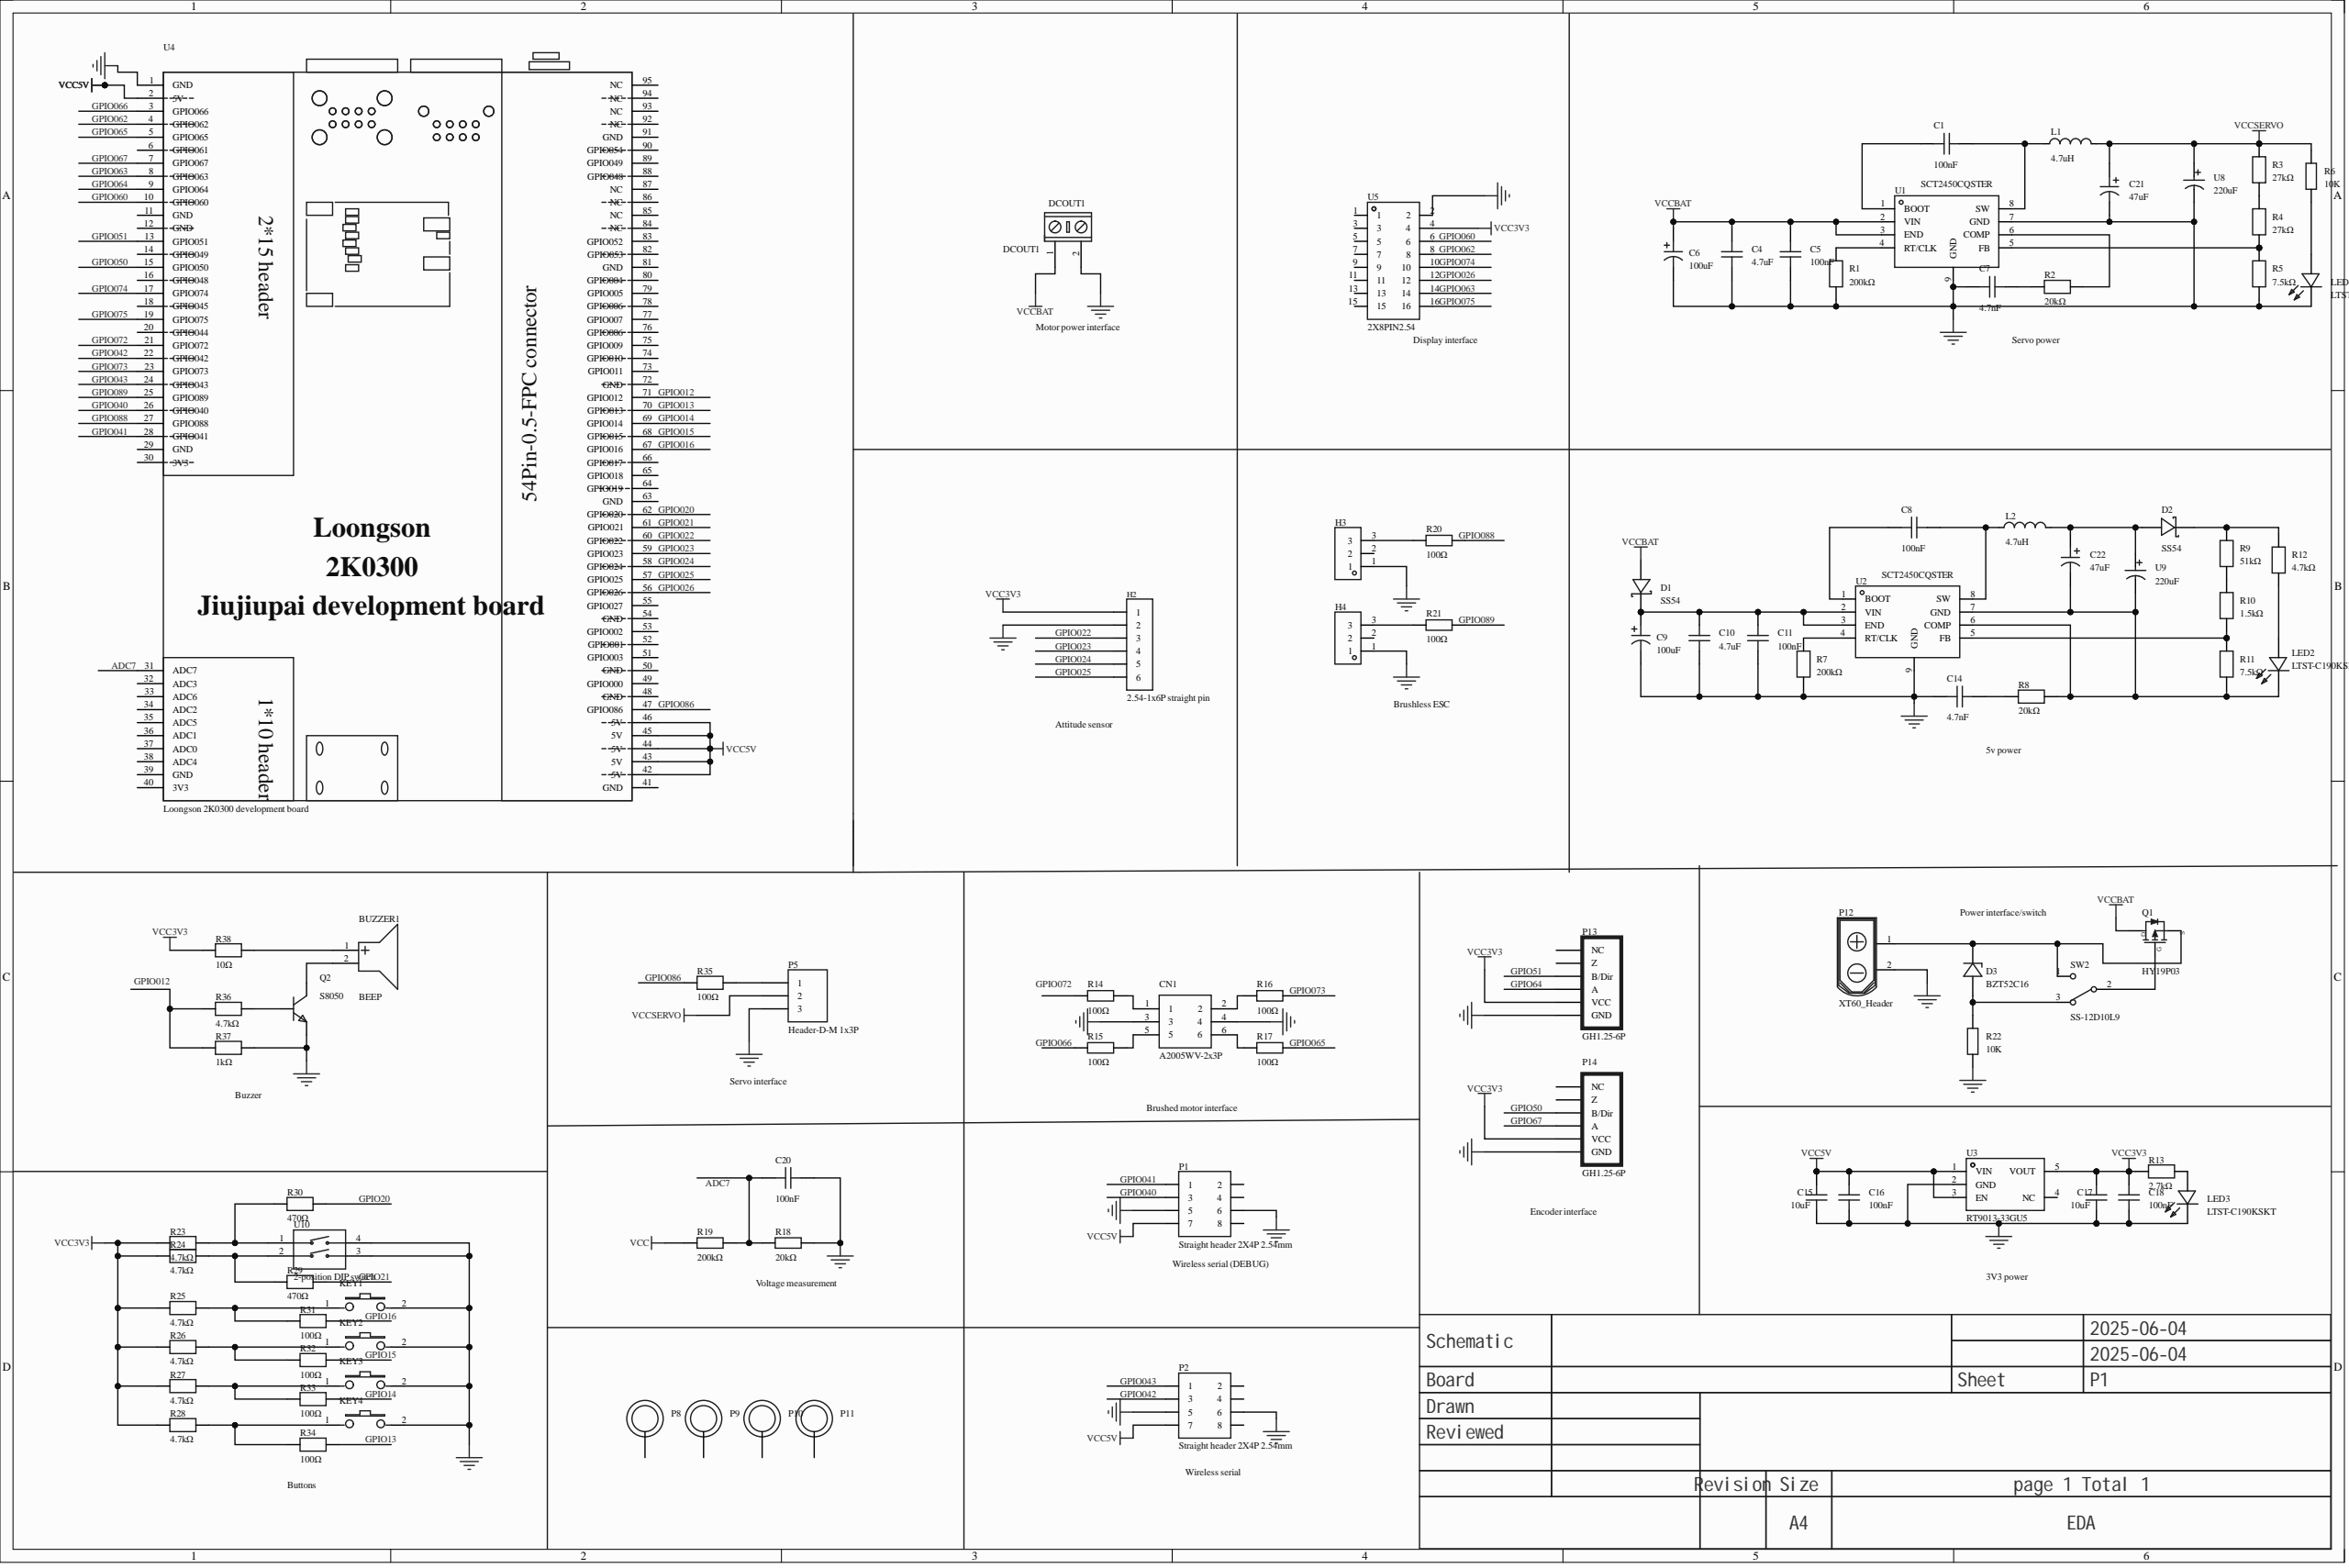Circuit board | Altium Designer | 94 parts | 61 nets
Bill of materials:
Comment,Description,Designator,Footprint,LibRef,Quantity
"BEEP","","BUZZER1","BUZ-TH_BD9-P50-D0.6-FD","BEEP","1"
"100nF","Capacitance:100nF;Tolerance:±10%;Rated voltage:100V;Temp coefficient:X7R;, [NoValue]","C1, C5, C8, C11, C16, C18, C20","C0603","06031C104K4T2A, CAP_0603","7"
"4.7uF","Capacitance:4.7uF;Tolerance:±20%;Rated voltage:16V;Temp coefficient:X5R;","C4, C10","C0402","0402X475M160NT","2"
"100uF","Capacitance:100uF;Tolerance:±20%;Rated voltage:8V;Equivalent series resistance (ESR):35mΩ@100kHz;","C6, C9","CAP-SMD_L3.5-W2.8-R-RD","8TPE100MAZB","2"
"4.7nF","Capacitance:4.7nF;Tolerance:±5%;Rated voltage:50V;Temp coefficient:C0G;","C7, C14","C0603","0603CG472J500NT","2"
"10uF","Capacitance:10uF;Tolerance:±10%;Rated voltage:10V;Temp coefficient:X7R;","C15, C17","C0805","C0805X106K8RACAUTO","2"
"47uF","Capacitance:47uF;Tolerance:±20%;Rated voltage:16V;Type:Polymer;","C21, C22","CAP-SMD_BD6.3-L6.6-W6.6-LS7.3-FD","SPT1CM470E05TRVZC","2"
"A2005WV-2x3P","间距:2mm;总PIN位数:6;排数:2;插针结构:2x3P;行距:2mm;安装类型:直插;圆针/方针:方针;额定电流:-;额定电压:-;配合针长度:4mm;塑高:-;端接针长度:2.8mm;触头材质:黄铜;触头镀层:金;工作温度范围:-40℃~+105℃;颜色:黑色;","CN1","HDR-TH_6P-P2.00-V-M-R2-C3-S2.00","A2005WV-2x3P","1"
"SS54","Diode configuration:Single;Forward voltage drop (Vf):550mV@5A;DC reverse voltage (Vr):40V;Rectified current:5A;","D1, D2","SMA_L4.4-W2.8-LS5.4-R-RD","SS54_C22452","2"
"BZT52C16","","D3","SOD-123-L","BZT52C16","1"
"DCOUT1","","DCOUT1","KF/WJ/DG 301-2P-5.0MM","DCOUT1","1"
"2.54-1x6P straight pin","间距:2.54mm;总PIN位数:6;排数:1;插针结构:1x6P;行距:-;安装类型:直插;圆针/方针:方针;额定电流:3A;额定电压:-;配合针长度:-;塑高:-;触头材质:黄铜;触头镀层:-;工作温度范围:-40℃~+105℃;颜色:黑色;","H2","HDR-TH_6P-P2.54-V-M-1","2.54-1x6P直针","1"
"","","H3, H4","HDR-TH_3P-P2.54-V-M","HDR-M_2.54_1x3P","2"
"Tact switch 3x6x2.5mm","","KEY1, KEY2, KEY3, KEY4","SW-SMD_L6.0-W3.6-LS8.0","轻触按键 3x6x2.5mm","4"
"4.7uH","Inductance:4.7uH;Tolerance:±20%;Rated current:6A;Saturation current (Isat):9A;Type:Molded inductor;","L1, L2","IND-SMD_L7.0-W6.6_VCMT063T","ZEMS0603-4R7M","2"
"LTST-C190KSKT","发光颜色:黄色;正向电压(VF):2.1V;功率:75mW;正向电流:20mA;主波长:584.5nm~597nm;二极管配置:-;透镜颜色:无色透明透镜;色温:-;发光强度:104mcd;发光角度:130°;载带方式:-;工作温度:-30℃~+85℃;","LED1, LED2, LED3","LED0603-RD","LTST-C190KSKT","3"
"Straight header 2X4P 2.54mm","Rows:-;Round/square pin:-;Rated current:-;Rated voltage:-;Mating pin length:-;Plastic height:-;Contact material:-;","P1, P2","HDR-TH_8P-P2.54-V-M-R2-C4-S2.54","直排针2X4P 2.54mm","2"
"Header-D-M 1x3P","1x3pin, through-hole, pin header","P5","HDR1X3-M","Header-D-M 1x3P","1"
"","","P8, P9, P10, P11","定位孔","定位孔","4"
"XT60_Header","XT60_Header","P12","Wired T-Header ThroughHole","XT60_Header","1"
"GH1.25-6P","COMPANY_A 1024-line encoder GH1.25-6P, board side","P13, P14","ECD-GH1.25-6P-SH","GH1.25-6P","2"
"HY19P03","","Q1","TO-252AA","HY19P03","1"
"S8050","","Q2","SOT-23(SOT-23-3)","S8050","1"
"200kΩ","","R1, R7, R19","R0603","AF0805FR-07200KL, RS-05K204JT","3"
"20kΩ","","R2, R8, R18","R0603","MMA02040D2002FB300, PTFR0805B20K0N9","3"
"27kΩ","Resistor type:Thin film resistor;Resistance:27kΩ;Tolerance:±0.1%;Power:125mW;Temp coefficient:±50ppm/?;","R3, R4","R0603","RT0805BRE0727KL","2"
"7.5kΩ","Resistor type:Thick film resistor;Resistance:7.5kΩ;Tolerance:±0.1%;Power:250mW;Working voltage:200V;Temp coefficient:±50ppm/?;","R5, R11","R0603","ERJ-PB3B7501V","2"
"10K","","R6, R22","R0603","Res_0402, Res_0603","2"
"51kΩ","Resistor type:Thin film resistor;Resistance:51kΩ;Tolerance:±0.1%;Power:63mW;Temp coefficient:±50ppm/?;","R9","R0603","RT0402BRE0751KL","1"
"1.5kΩ","Resistor type:Thin film resistor;Resistance:1.5kΩ;Tolerance:±0.1%;Power:100mW;Max working voltage:150V;Temp coefficient:±25ppm/?;","R10","R0603","RGT2012P-152-B-T5","1"
"4.7kΩ","Resistor type:Thin film resistor;Resistance:4.7kΩ;Tolerance:±1%;Power:400mW;Temp coefficient:±50ppm/?;","R12, R23, R24, R25, R26, R27, R28, R36","R0603","MMA02040C4701FB300","8"
"2.7kΩ","Resistor type:Thick film resistor;Resistance:2.7kΩ;Tolerance:±1%;Power:750mW;Working voltage:200V;Temp coefficient:±100ppm/?;","R13","R0603","CRCW12062K70FKEAHP","1"
"100Ω","","R14, R15, R16, R17, R20, R21, R31, R32, R33, R34, R35","R0603","RS-05K1000FT, PTFR1206B100RV9","11"
"470Ω","Resistor type:Thick film resistor;Resistance:470Ω;Tolerance:±1%;Power:62.5mW;Working voltage:50V;Temp coefficient:±100ppm/?;","R29, R30","R0603","FRC0402F4700TS","2"
"1kΩ","Resistor type:Thin film resistor;Resistance:1kΩ;Tolerance:±1%;Power:1W;Working voltage:350V;Temp coefficient:±50ppm/?;","R37","R0603","MMB02070C1001FB200","1"
"10Ω","Resistance:10Ω;Tolerance:±5%;Power:62.5mW;","R38","R0603","RCA0210RJLF","1"
"SS-12D10L9","","SW2","MTS-10x","单刀双掷开关","1"
"SCT2450CQSTER","","U1, U2","ESOP-8_L4.9-W3.9-P1.27-LS6.0-BL-EP","SCT2450CQSTER","2"
"RT9013-33GU5","Output type:Fixed;Max input voltage:5.5V;Output voltage:3.3V;Output current:500mA;Power supply rejection ratio (PSRR):50dB@(10kHz);Output polarity:Positive;","U3","SC-70-5_L2.0-W1.3-P0.65-LS2.1-BR","RT9013-33GU5","1"
"Loongson 2K0300 development board","COMPANY_A Loongson 2K0300 Jiujiupai development board full schematic, ready to use","U4","龙芯2K0300久久派开发板","龙芯2K0300久久派开发板","1"
"2X8PIN2.54","","U5","HDR-TH_16P-P2.54-V-M-R2-C8-S2.54","2X8PIN2.54","1"
"220uF","","U8, U9","CAP-SMD_BD6.3-L6.6-W6.6-LS7.2-FD","220uF","2"
"2-position DIP switch","","U10","SW-TH_4P-L9.9-W6.8-P7.62-BL","2位DIP拨码开关","1"
Netlist (Protel format):
[
BUZZER1
BUZ-TH_BD9-P50-D0.6-FD
BEEP



]
[
C1
C0603
100nF



]
[
C4
C0402
4.7uF



]
[
C5
C0603
100nF



]
[
C6
CAP-SMD_L3.5-W2.8-R-RD
100uF



]
[
C7
C0603
4.7nF



]
[
C8
C0603
100nF



]
[
C9
CAP-SMD_L3.5-W2.8-R-RD
100uF



]
[
C10
C0402
4.7uF



]
[
C11
C0603
100nF



]
[
C14
C0603
4.7nF



]
[
C15
C0805
10uF



]
[
C16
C0603
100nF



]
[
C17
C0805
10uF



]
[
C18
C0603
100nF



]
[
C20
C0603
100nF



]
[
C21
CAP-SMD_BD6.3-L6.6-W6.6-LS7.3-FD
47uF



]
[
C22
CAP-SMD_BD6.3-L6.6-W6.6-LS7.3-FD
47uF



]
[
CN1
HDR-TH_6P-P2.00-V-M-R2-C3-S2.00
A2005WV-2x3P



]
[
D1
SMA_L4.4-W2.8-LS5.4-R-RD
SS54



]
[
D2
SMA_L4.4-W2.8-LS5.4-R-RD
SS54



]
[
D3
SOD-123-L
BZT52C16



]
[
DCOUT1
KF/WJ/DG 301-2P-5.0MM
DCOUT1



]
[
H2
HDR-TH_6P-P2.54-V-M-1
2.54-1x6P straight pin



]
[
H3
HDR-TH_3P-P2.54-V-M




]
[
H4
HDR-TH_3P-P2.54-V-M




]
[
KEY1
SW-SMD_L6.0-W3.6-LS8.0
Tact switch 3x6x2.5mm



]
[
KEY2
SW-SMD_L6.0-W3.6-LS8.0
Tact switch 3x6x2.5mm



]
[
KEY3
SW-SMD_L6.0-W3.6-LS8.0
Tact switch 3x6x2.5mm



]
[
KEY4
SW-SMD_L6.0-W3.6-LS8.0
Tact switch 3x6x2.5mm



]
[
L1
IND-SMD_L7.0-W6.6_VCMT063T
4.7uH



]
[
L2
IND-SMD_L7.0-W6.6_VCMT063T
4.7uH



]
[
LED1
LED0603-RD
LTST-C190KSKT



]
[
LED2
LED0603-RD
LTST-C190KSKT



]
[
LED3
LED0603-RD
LTST-C190KSKT



]
[
P1
HDR-TH_8P-P2.54-V-M-R2-C4-S2.54
Straight header 2X4P 2.54mm



]
[
P2
HDR-TH_8P-P2.54-V-M-R2-C4-S2.54
Straight header 2X4P 2.54mm



]
[
P5
HDR1X3-M
Header-D-M 1x3P



]
[
P8
定位孔




]
[
P9
定位孔




]
[
P10
定位孔




]
[
P11
定位孔




]
[
P12
Wired T-Header ThroughHole
XT60_Header



]
[
P13
ECD-GH1.25-6P-SH
GH1.25-6P



]
[
P14
ECD-GH1.25-6P-SH
GH1.25-6P



]
[
Q1
TO-252AA
HY19P03



]
[
Q2
SOT-23(SOT-23-3)
S8050



]
[
R1
R0603
200kΩ



]
[
R2
R0603
20kΩ



]
[
R3
R0603
27kΩ



]
[
R4
R0603
27kΩ



]
[
R5
R0603
7.5kΩ



]
[
R6
R0603
10K



]
[
R7
R0603
200kΩ



]
[
R8
R0603
20kΩ



]
[
R9
R0603
51kΩ



]
[
R10
R0603
1.5kΩ



]
[
R11
R0603
7.5kΩ



]
[
R12
R0603
4.7kΩ



]
[
R13
R0603
2.7kΩ



]
[
R14
R0603
100Ω



]
[
R15
R0603
100Ω



]
[
R16
R0603
100Ω



]
[
R17
R0603
100Ω



]
[
R18
R0603
20kΩ



]
[
R19
R0603
200kΩ



]
[
R20
R0603
100Ω



]
[
R21
R0603
100Ω



]
[
R22
R0603
10K



]
[
R23
R0603
4.7kΩ



]
[
R24
R0603
4.7kΩ



]
[
R25
R0603
4.7kΩ



]
[
R26
R0603
4.7kΩ



]
[
R27
R0603
4.7kΩ



]
[
R28
R0603
4.7kΩ



]
[
R29
R0603
470Ω



]
[
R30
R0603
470Ω



]
[
R31
R0603
100Ω



]
[
R32
R0603
100Ω



]
[
R33
R0603
100Ω



]
[
R34
R0603
100Ω



]
[
R35
R0603
100Ω



]
[
R36
R0603
4.7kΩ



]
[
R37
R0603
1kΩ



]
[
R38
R0603
10Ω



]
[
SW2
MTS-10x
SS-12D10L9



]
[
U1
ESOP-8_L4.9-W3.9-P1.27-LS6.0-BL-EP
SCT2450CQSTER



]
[
U2
ESOP-8_L4.9-W3.9-P1.27-LS6.0-BL-EP
SCT2450CQSTER



]
[
U3
SC-70-5_L2.0-W1.3-P0.65-LS2.1-BR
RT9013-33GU5



]
[
U4
龙芯2K0300久久派开发板
Loongson 2K0300 development board



]
[
U5
HDR-TH_16P-P2.54-V-M-R2-C8-S2.54
2X8PIN2.54



]
[
U8
CAP-SMD_BD6.3-L6.6-W6.6-LS7.2-FD
220uF



]
[
U9
CAP-SMD_BD6.3-L6.6-W6.6-LS7.2-FD
220uF



]
[
U10
SW-TH_4P-L9.9-W6.8-P7.62-BL
2-position DIP switch



]
(
VCCSERVO
C21-1
L1-2
P5-2
R3-2
R6-2
U8-1
)
(
VCCBAT
C4-2
C5-2
C6-1
D1-1
DCOUT1-1
Q1-1
U1-2
U1-3
)
(
VCC5V
C15-2
C16-2
P1-7
P2-7
U3-1
U3-3
U4-2
U4-42
U4-43
U4-44
U4-45
U4-46
)
(
VCC3V3
C17-2
C18-2
H2-1
P13-2
P14-2
R13-1
R23-1
R24-1
R25-1
R26-1
R27-1
R28-1
R38-1
U3-5
U5-4
)
(
NetR36_1
R36-1
R37-1
)
(
NetR24_2
R24-2
R29-1
U10-2
)
(
NetR23_2
R23-2
R30-1
U10-1
)
(
NetR10_1
R10-1
R11-2
U2-5
)
(
NetR9_1
R9-1
R10-2
)
(
NetR7_2
R7-2
U2-4
)
(
NetR4_1
R4-1
R5-2
U1-5
)
(
NetR3_1
R3-1
R4-2
)
(
NetR2_1
R2-1
U1-6
)
(
NetR1_2
R1-2
U1-4
)
(
NetQ2_1
Q2-1
R36-2
)
(
NetQ1_2
Q1-2
SW2-2
)
(
NetP5_1
P5-1
R35-2
)
(
NetLED3_2
LED3-2
R13-2
)
(
NetLED2_2
LED2-2
R12-1
)
(
NetLED1_2
LED1-2
R6-1
)
(
NetKEY4_1
KEY4-1
R28-2
R34-1
)
(
NetKEY3_1
KEY3-1
R27-2
R33-1
)
(
NetKEY2_1
KEY2-1
R26-2
R32-1
)
(
NetKEY1_1
KEY1-1
R25-2
R31-1
)
(
NetH4_3
H4-3
R21-1
)
(
NetH3_3
H3-3
R20-1
)
(
NetD3_K
D3-K
P12-1
Q1-3
SW2-1
)
(
NetD3_A
D3-A
R22-2
SW2-3
)
(
NetD2_2
D2-2
R9-2
R12-2
)
(
NetCN1_6
CN1-6
R17-1
)
(
NetCN1_5
CN1-5
R15-2
)
(
NetCN1_2
CN1-2
R16-1
)
(
NetCN1_1
CN1-1
R14-2
)
(
NetC22_2
C22-2
LED2-1
R8-1
R11-1
U2-6
U2-7
U9-2
)
(
NetC22_1
C22-1
D2-1
L2-2
U9-1
)
(
NetC14_2
C14-2
R8-2
)
(
NetC9_1
C9-1
C10-2
C11-2
D1-2
U2-2
U2-3
)
(
NetC8_2
C8-2
L2-1
U2-8
)
(
NetC8_1
C8-1
U2-1
)
(
NetC7_2
C7-2
R2-2
)
(
NetC1_2
C1-2
L1-1
U1-8
)
(
NetC1_1
C1-1
U1-1
)
(
NetBUZZER1_2
BUZZER1-2
Q2-3
)
(
NetBUZZER1_1
BUZZER1-1
R38-2
)
(
GPIO086
R35-1
U4-47
)
(
GPIO075
U4-19
U5-16
)
(
GPIO074
U4-17
U5-10
)
(
GPIO063
U4-8
U5-14
)
(
GPIO062
U4-4
U5-8
)
(
GPIO060
U4-10
U5-6
)
(
GPIO043
P2-1
U4-24
)
(
GPIO042
P2-3
U4-22
)
(
GPIO041
P1-1
U4-28
)
(
GPIO040
P1-3
U4-26
)
(
GPIO026
U4-56
U5-12
)
(
GPIO025
H2-6
U4-57
)
(
GPIO024
H2-5
U4-58
)
(
GPIO023
H2-4
U4-59
)
(
GPIO022
H2-3
U4-60
)
(
GND
C4-1
C5-1
C6-2
C7-1
C9-2
C10-1
C11-1
C14-1
C15-1
C16-1
C17-1
C18-1
C20-2
C21-2
CN1-3
CN1-4
DCOUT1-2
H2-2
H3-1
H4-1
KEY1-2
KEY2-2
KEY3-2
KEY4-2
LED1-1
LED3-1
P1-5
P1-6
P2-5
P2-6
P5-3
P12-2
P13-1
P14-1
Q2-2
R1-1
R5-1
R7-1
R18-2
R22-1
R37-2
U1-7
U1-9
U2-9
U3-2
U4-1
U5-2
U8-2
U10-3
U10-4
)
(
ADC7
C20-1
R18-1
R19-2
U4-31
)